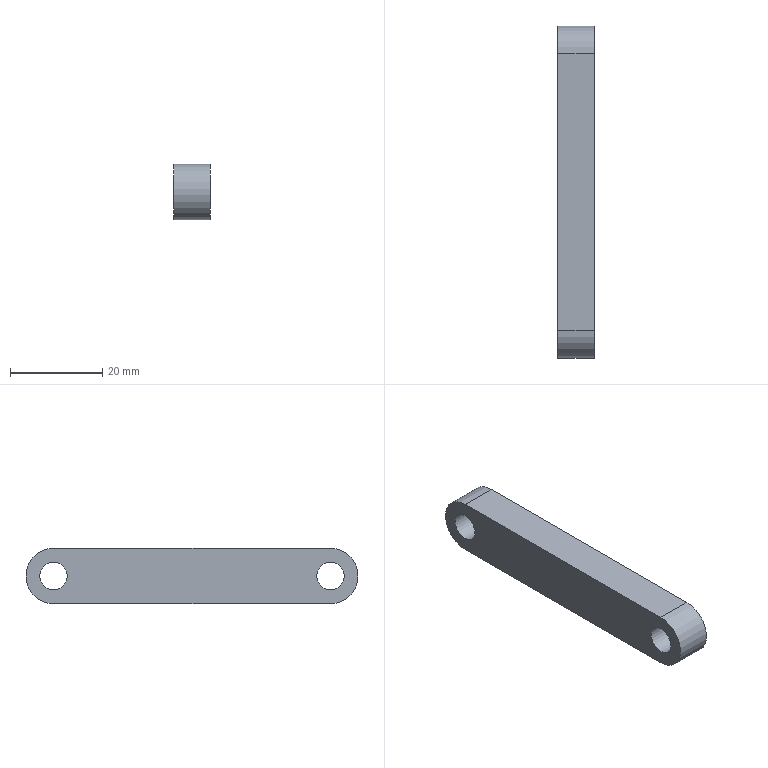Part | NX | features OFFSET_REGION 3, DATUM_CSYS 2, EXTRUDE 1, SKETCH 1 | 1 solid | 8 faces | box 8 x 72 x 12 mm | volume 6212 mm3 | cylinder 4 | plane 4 | commonest cylinder face diameters 6 x2 12 x2
STEP:
#1=CARTESIAN_POINT('',(0.,-30.,6.));
#2=VERTEX_POINT('',#1);
#3=CARTESIAN_POINT('',(0.,-30.,-6.));
#4=VERTEX_POINT('',#3);
#5=CARTESIAN_POINT('',(0.,-30.,0.));
#6=DIRECTION('',(1.,0.,0.));
#7=DIRECTION('',(0.,0.,-1.));
#8=AXIS2_PLACEMENT_3D('',#5,#6,#7);
#9=CIRCLE('',#8,6.);
#10=EDGE_CURVE('',#2,#4,#9,.T.);
#11=ORIENTED_EDGE('',*,*,#10,.T.);
#12=CARTESIAN_POINT('',(8.,-30.,-6.));
#13=VERTEX_POINT('',#12);
#14=CARTESIAN_POINT('',(8.,-30.,-6.));
#15=DIRECTION('',(1.,0.,0.));
#16=VECTOR('',#15,1000.);
#17=LINE('',#14,#16);
#18=EDGE_CURVE('',#13,#4,#17,.F.);
#19=ORIENTED_EDGE('',*,*,#18,.F.);
#20=CARTESIAN_POINT('',(8.,-30.,6.));
#21=VERTEX_POINT('',#20);
#22=CARTESIAN_POINT('',(8.,-30.,0.));
#23=DIRECTION('',(1.,0.,0.));
#24=DIRECTION('',(0.,0.,-1.));
#25=AXIS2_PLACEMENT_3D('',#22,#23,#24);
#26=CIRCLE('',#25,6.);
#27=EDGE_CURVE('',#21,#13,#26,.T.);
#28=ORIENTED_EDGE('',*,*,#27,.F.);
#29=CARTESIAN_POINT('',(8.,-30.,6.));
#30=DIRECTION('',(-1.,0.,0.));
#31=VECTOR('',#30,1000.);
#32=LINE('',#29,#31);
#33=EDGE_CURVE('',#21,#2,#32,.T.);
#34=ORIENTED_EDGE('',*,*,#33,.T.);
#35=EDGE_LOOP('',(#11,#19,#28,#34));
#36=FACE_BOUND('',#35,.T.);
#37=CARTESIAN_POINT('',(8.,-30.,0.));
#38=DIRECTION('',(-1.,0.,0.));
#39=DIRECTION('',(0.,0.,1.));
#40=AXIS2_PLACEMENT_3D('',#37,#38,#39);
#41=CYLINDRICAL_SURFACE('',#40,6.);
#42=ADVANCED_FACE('',(#36),#41,.T.);
#43=CARTESIAN_POINT('',(0.,30.,-6.));
#44=VERTEX_POINT('',#43);
#45=CARTESIAN_POINT('',(0.,-30.,-6.));
#46=DIRECTION('',(0.,1.,0.));
#47=VECTOR('',#46,1000.);
#48=LINE('',#45,#47);
#49=EDGE_CURVE('',#4,#44,#48,.T.);
#50=ORIENTED_EDGE('',*,*,#49,.T.);
#51=CARTESIAN_POINT('',(8.,30.,-6.));
#52=VERTEX_POINT('',#51);
#53=CARTESIAN_POINT('',(8.,30.,-6.));
#54=DIRECTION('',(-1.,0.,0.));
#55=VECTOR('',#54,1000.);
#56=LINE('',#53,#55);
#57=EDGE_CURVE('',#52,#44,#56,.T.);
#58=ORIENTED_EDGE('',*,*,#57,.F.);
#59=CARTESIAN_POINT('',(8.,-30.,-6.));
#60=DIRECTION('',(0.,1.,0.));
#61=VECTOR('',#60,1000.);
#62=LINE('',#59,#61);
#63=EDGE_CURVE('',#13,#52,#62,.T.);
#64=ORIENTED_EDGE('',*,*,#63,.F.);
#65=ORIENTED_EDGE('',*,*,#18,.T.);
#66=EDGE_LOOP('',(#50,#58,#64,#65));
#67=FACE_BOUND('',#66,.T.);
#68=CARTESIAN_POINT('',(8.,-30.,-6.));
#69=DIRECTION('',(0.,0.,1.));
#70=DIRECTION('',(1.,0.,0.));
#71=AXIS2_PLACEMENT_3D('',#68,#69,#70);
#72=PLANE('',#71);
#73=ADVANCED_FACE('',(#67),#72,.F.);
#74=CARTESIAN_POINT('',(0.,30.,6.));
#75=VERTEX_POINT('',#74);
#76=CARTESIAN_POINT('',(0.,30.,0.));
#77=DIRECTION('',(1.,0.,0.));
#78=DIRECTION('',(0.,0.,-1.));
#79=AXIS2_PLACEMENT_3D('',#76,#77,#78);
#80=CIRCLE('',#79,6.);
#81=EDGE_CURVE('',#44,#75,#80,.T.);
#82=ORIENTED_EDGE('',*,*,#81,.T.);
#83=CARTESIAN_POINT('',(8.,30.,6.));
#84=VERTEX_POINT('',#83);
#85=CARTESIAN_POINT('',(8.,30.,6.));
#86=DIRECTION('',(-1.,0.,0.));
#87=VECTOR('',#86,1000.);
#88=LINE('',#85,#87);
#89=EDGE_CURVE('',#84,#75,#88,.T.);
#90=ORIENTED_EDGE('',*,*,#89,.F.);
#91=CARTESIAN_POINT('',(8.,30.,0.));
#92=DIRECTION('',(1.,0.,0.));
#93=DIRECTION('',(0.,0.,-1.));
#94=AXIS2_PLACEMENT_3D('',#91,#92,#93);
#95=CIRCLE('',#94,6.);
#96=EDGE_CURVE('',#52,#84,#95,.T.);
#97=ORIENTED_EDGE('',*,*,#96,.F.);
#98=ORIENTED_EDGE('',*,*,#57,.T.);
#99=EDGE_LOOP('',(#82,#90,#97,#98));
#100=FACE_BOUND('',#99,.T.);
#101=CARTESIAN_POINT('',(8.,30.,0.));
#102=DIRECTION('',(-1.,0.,0.));
#103=DIRECTION('',(0.,0.,1.));
#104=AXIS2_PLACEMENT_3D('',#101,#102,#103);
#105=CYLINDRICAL_SURFACE('',#104,6.);
#106=ADVANCED_FACE('',(#100),#105,.T.);
#107=CARTESIAN_POINT('',(8.,-30.,-3.));
#108=VERTEX_POINT('',#107);
#109=CARTESIAN_POINT('',(8.,-30.,0.));
#110=DIRECTION('',(1.,0.,0.));
#111=DIRECTION('',(0.,0.,-1.));
#112=AXIS2_PLACEMENT_3D('',#109,#110,#111);
#113=CIRCLE('',#112,3.);
#114=EDGE_CURVE('',#108,#108,#113,.T.);
#115=ORIENTED_EDGE('',*,*,#114,.T.);
#116=EDGE_LOOP('',(#115));
#117=FACE_BOUND('',#116,.T.);
#118=CARTESIAN_POINT('',(0.,-30.,-3.));
#119=VERTEX_POINT('',#118);
#120=CARTESIAN_POINT('',(0.,-30.,0.));
#121=DIRECTION('',(1.,0.,0.));
#122=DIRECTION('',(0.,0.,-1.));
#123=AXIS2_PLACEMENT_3D('',#120,#121,#122);
#124=CIRCLE('',#123,3.);
#125=EDGE_CURVE('',#119,#119,#124,.T.);
#126=ORIENTED_EDGE('',*,*,#125,.F.);
#127=EDGE_LOOP('',(#126));
#128=FACE_BOUND('',#127,.T.);
#129=CARTESIAN_POINT('',(8.,-30.,0.));
#130=DIRECTION('',(-1.,0.,0.));
#131=DIRECTION('',(0.,0.,1.));
#132=AXIS2_PLACEMENT_3D('',#129,#130,#131);
#133=CYLINDRICAL_SURFACE('',#132,3.);
#134=ADVANCED_FACE('',(#117,#128),#133,.F.);
#135=CARTESIAN_POINT('',(0.,30.,6.));
#136=DIRECTION('',(0.,-1.,0.));
#137=VECTOR('',#136,1000.);
#138=LINE('',#135,#137);
#139=EDGE_CURVE('',#75,#2,#138,.T.);
#140=ORIENTED_EDGE('',*,*,#139,.T.);
#141=ORIENTED_EDGE('',*,*,#33,.F.);
#142=CARTESIAN_POINT('',(8.,30.,6.));
#143=DIRECTION('',(0.,-1.,0.));
#144=VECTOR('',#143,1000.);
#145=LINE('',#142,#144);
#146=EDGE_CURVE('',#84,#21,#145,.T.);
#147=ORIENTED_EDGE('',*,*,#146,.F.);
#148=ORIENTED_EDGE('',*,*,#89,.T.);
#149=EDGE_LOOP('',(#140,#141,#147,#148));
#150=FACE_BOUND('',#149,.T.);
#151=CARTESIAN_POINT('',(8.,30.,6.));
#152=DIRECTION('',(0.,0.,-1.));
#153=DIRECTION('',(-1.,0.,0.));
#154=AXIS2_PLACEMENT_3D('',#151,#152,#153);
#155=PLANE('',#154);
#156=ADVANCED_FACE('',(#150),#155,.F.);
#157=CARTESIAN_POINT('',(8.,30.,-3.));
#158=VERTEX_POINT('',#157);
#159=CARTESIAN_POINT('',(8.,30.,0.));
#160=DIRECTION('',(1.,0.,0.));
#161=DIRECTION('',(0.,0.,-1.));
#162=AXIS2_PLACEMENT_3D('',#159,#160,#161);
#163=CIRCLE('',#162,3.);
#164=EDGE_CURVE('',#158,#158,#163,.T.);
#165=ORIENTED_EDGE('',*,*,#164,.T.);
#166=EDGE_LOOP('',(#165));
#167=FACE_BOUND('',#166,.T.);
#168=CARTESIAN_POINT('',(0.,30.,-3.));
#169=VERTEX_POINT('',#168);
#170=CARTESIAN_POINT('',(0.,30.,0.));
#171=DIRECTION('',(1.,0.,0.));
#172=DIRECTION('',(0.,0.,-1.));
#173=AXIS2_PLACEMENT_3D('',#170,#171,#172);
#174=CIRCLE('',#173,3.);
#175=EDGE_CURVE('',#169,#169,#174,.T.);
#176=ORIENTED_EDGE('',*,*,#175,.F.);
#177=EDGE_LOOP('',(#176));
#178=FACE_BOUND('',#177,.T.);
#179=CARTESIAN_POINT('',(8.,30.,0.));
#180=DIRECTION('',(-1.,0.,0.));
#181=DIRECTION('',(0.,0.,1.));
#182=AXIS2_PLACEMENT_3D('',#179,#180,#181);
#183=CYLINDRICAL_SURFACE('',#182,3.);
#184=ADVANCED_FACE('',(#167,#178),#183,.F.);
#185=ORIENTED_EDGE('',*,*,#27,.T.);
#186=ORIENTED_EDGE('',*,*,#63,.T.);
#187=ORIENTED_EDGE('',*,*,#96,.T.);
#188=ORIENTED_EDGE('',*,*,#146,.T.);
#189=EDGE_LOOP('',(#185,#186,#187,#188));
#190=FACE_BOUND('',#189,.T.);
#191=ORIENTED_EDGE('',*,*,#114,.F.);
#192=EDGE_LOOP('',(#191));
#193=FACE_BOUND('',#192,.T.);
#194=ORIENTED_EDGE('',*,*,#164,.F.);
#195=EDGE_LOOP('',(#194));
#196=FACE_BOUND('',#195,.T.);
#197=CARTESIAN_POINT('',(8.,-30.,0.));
#198=DIRECTION('',(1.,0.,0.));
#199=DIRECTION('',(0.,0.,-1.));
#200=AXIS2_PLACEMENT_3D('',#197,#198,#199);
#201=PLANE('',#200);
#202=ADVANCED_FACE('',(#190,#193,#196),#201,.T.);
#203=ORIENTED_EDGE('',*,*,#10,.F.);
#204=ORIENTED_EDGE('',*,*,#139,.F.);
#205=ORIENTED_EDGE('',*,*,#81,.F.);
#206=ORIENTED_EDGE('',*,*,#49,.F.);
#207=EDGE_LOOP('',(#203,#204,#205,#206));
#208=FACE_BOUND('',#207,.T.);
#209=ORIENTED_EDGE('',*,*,#125,.T.);
#210=EDGE_LOOP('',(#209));
#211=FACE_BOUND('',#210,.T.);
#212=ORIENTED_EDGE('',*,*,#175,.T.);
#213=EDGE_LOOP('',(#212));
#214=FACE_BOUND('',#213,.T.);
#215=CARTESIAN_POINT('',(0.,-30.,0.));
#216=DIRECTION('',(1.,0.,0.));
#217=DIRECTION('',(0.,0.,-1.));
#218=AXIS2_PLACEMENT_3D('',#215,#216,#217);
#219=PLANE('',#218);
#220=ADVANCED_FACE('',(#208,#211,#214),#219,.F.);
#221=CLOSED_SHELL('',(#42,#73,#106,#134,#156,#184,#202,#220));
#222=MANIFOLD_SOLID_BREP('',#221);
#223=(LENGTH_UNIT()NAMED_UNIT(*)SI_UNIT(.MILLI.,.METRE.));
#224=UNCERTAINTY_MEASURE_WITH_UNIT(LENGTH_MEASURE(0.00001),#223,'','');
#225=(NAMED_UNIT(*)PLANE_ANGLE_UNIT()SI_UNIT($,.RADIAN.));
#226=(NAMED_UNIT(*)SI_UNIT($,.STERADIAN.)SOLID_ANGLE_UNIT());
#227=(GEOMETRIC_REPRESENTATION_CONTEXT(3)GLOBAL_UNCERTAINTY_ASSIGNED_CONTEXT((#224))GLOBAL_UNIT_ASSIGNED_CONTEXT((#223,#225,#226))REPRESENTATION_CONTEXT('',''));
#228=ADVANCED_BREP_SHAPE_REPRESENTATION('',(#222),#227);